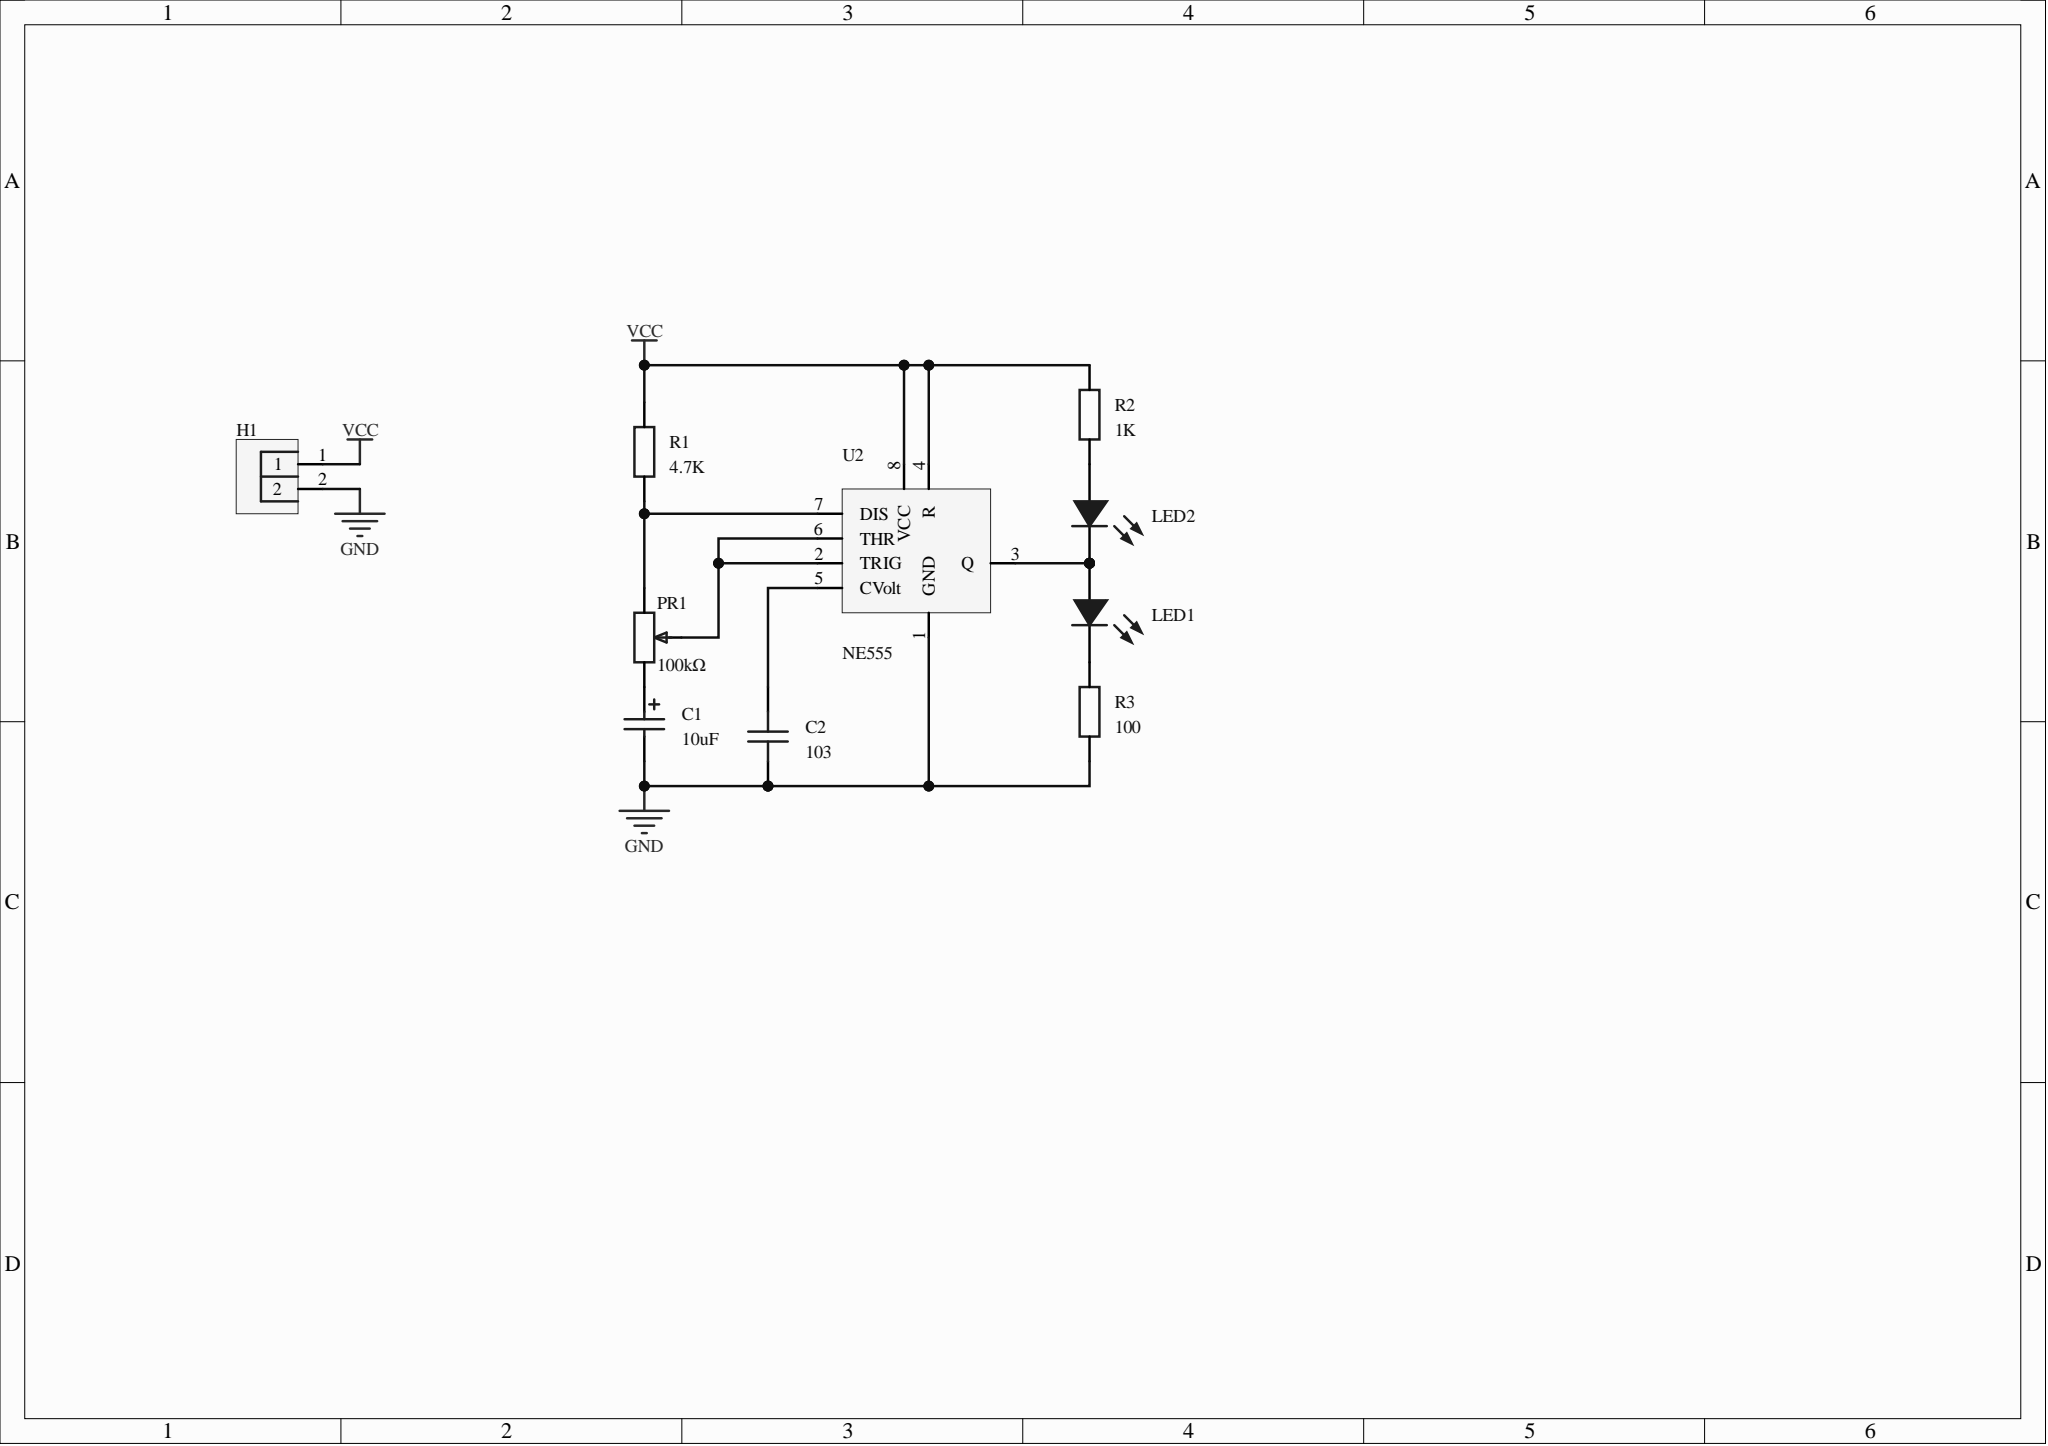Circuit board | Altium Designer | 10 parts | 9 nets
Bill of materials:
Comment,Description,Designator,Footprint,LibRef,Quantity
"10uF","","C1","C_Ele_SMD_3x5.4mm","C_Ele_SMD_3x5.4mm","1"
"103","","C2","C0603","CAP_0603","1"
"","","H1","HDR-TH_2P-P2.54-V-M-1","HDR-M_2.54_1x2P","1"
"","","LED1, LED2","LED_0603","LED_0603-B","2"
"100kΩ","","PR1","R_3296","R_3296","1"
"4.7K","","R1","R0603","Res_0603","1"
"1K","","R2","R0603","Res_0603","1"
"100","","R3","R0603","Res_0603","1"
"NE555","","U2","DIP-8_L9.8-W6.4-P2.54-LS7.6-BL","NE555","1"
Netlist (Protel format):
[
C1
C_Ele_SMD_3x5.4mm
10uF



]
[
C2
C0603
103



]
[
H1
HDR-TH_2P-P2.54-V-M-1




]
[
LED1
LED_0603




]
[
LED2
LED_0603




]
[
PR1
R_3296
100kΩ



]
[
R1
R0603
4.7K



]
[
R2
R0603
1K



]
[
R3
R0603
100



]
[
U2
DIP-8_L9.8-W6.4-P2.54-LS7.6-BL
NE555



]
(
VCC
H1-1
R1-2
R2-2
U2-4
U2-8
)
(
NetPR1_3
PR1-3
R1-1
U2-7
)
(
NetPR1_2
PR1-2
U2-2
U2-6
)
(
NetLED2_2
LED2-2
R2-1
)
(
NetLED1_2
LED1-2
LED2-1
U2-3
)
(
NetLED1_1
LED1-1
R3-2
)
(
NetC2_2
C2-2
U2-5
)
(
NetC1_1
C1-1
PR1-1
)
(
GND
C1-2
C2-1
H1-2
R3-1
U2-1
)